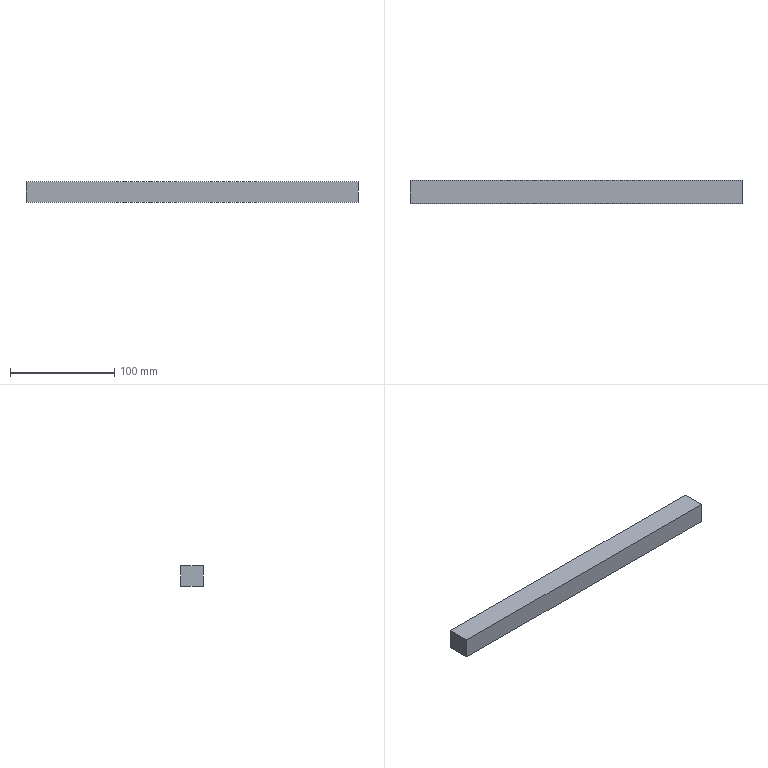Part | SolidWorks | features Extrusion 1 | 1 solid | 6 faces | box 318 x 22 x 20 mm | volume 139920 mm3 | plane 6
STEP:
#1=CARTESIAN_POINT('',(0.,22.,0.));
#2=VERTEX_POINT('',#1);
#3=CARTESIAN_POINT('',(0.,0.,0.));
#4=VERTEX_POINT('',#3);
#5=CARTESIAN_POINT('',(0.,0.,0.));
#6=DIRECTION('',(0.,-1.,0.));
#7=VECTOR('',#6,1000.);
#8=LINE('',#5,#7);
#9=EDGE_CURVE('',#2,#4,#8,.T.);
#10=ORIENTED_EDGE('',*,*,#9,.T.);
#11=CARTESIAN_POINT('',(0.,0.,20.));
#12=VERTEX_POINT('',#11);
#13=CARTESIAN_POINT('',(0.,0.,20.));
#14=DIRECTION('',(0.,0.,-1.));
#15=VECTOR('',#14,1000.);
#16=LINE('',#13,#15);
#17=EDGE_CURVE('',#12,#4,#16,.T.);
#18=ORIENTED_EDGE('',*,*,#17,.F.);
#19=CARTESIAN_POINT('',(0.,22.,20.));
#20=VERTEX_POINT('',#19);
#21=CARTESIAN_POINT('',(0.,0.,20.));
#22=DIRECTION('',(0.,-1.,0.));
#23=VECTOR('',#22,1000.);
#24=LINE('',#21,#23);
#25=EDGE_CURVE('',#20,#12,#24,.T.);
#26=ORIENTED_EDGE('',*,*,#25,.F.);
#27=CARTESIAN_POINT('',(0.,22.,20.));
#28=DIRECTION('',(0.,0.,-1.));
#29=VECTOR('',#28,1000.);
#30=LINE('',#27,#29);
#31=EDGE_CURVE('',#20,#2,#30,.T.);
#32=ORIENTED_EDGE('',*,*,#31,.T.);
#33=EDGE_LOOP('',(#10,#18,#26,#32));
#34=FACE_OUTER_BOUND('',#33,.T.);
#35=CARTESIAN_POINT('',(0.,0.,20.));
#36=DIRECTION('',(1.,0.,0.));
#37=DIRECTION('',(0.,0.,-1.));
#38=AXIS2_PLACEMENT_3D('',#35,#36,#37);
#39=PLANE('',#38);
#40=ADVANCED_FACE('',(#34),#39,.F.);
#41=CARTESIAN_POINT('',(318.,0.,0.));
#42=VERTEX_POINT('',#41);
#43=CARTESIAN_POINT('',(0.,0.,0.));
#44=DIRECTION('',(1.,0.,0.));
#45=VECTOR('',#44,1000.);
#46=LINE('',#43,#45);
#47=EDGE_CURVE('',#4,#42,#46,.T.);
#48=ORIENTED_EDGE('',*,*,#47,.T.);
#49=CARTESIAN_POINT('',(318.,0.,20.));
#50=VERTEX_POINT('',#49);
#51=CARTESIAN_POINT('',(318.,0.,20.));
#52=DIRECTION('',(0.,0.,-1.));
#53=VECTOR('',#52,1000.);
#54=LINE('',#51,#53);
#55=EDGE_CURVE('',#50,#42,#54,.T.);
#56=ORIENTED_EDGE('',*,*,#55,.F.);
#57=CARTESIAN_POINT('',(0.,0.,20.));
#58=DIRECTION('',(1.,0.,0.));
#59=VECTOR('',#58,1000.);
#60=LINE('',#57,#59);
#61=EDGE_CURVE('',#12,#50,#60,.T.);
#62=ORIENTED_EDGE('',*,*,#61,.F.);
#63=ORIENTED_EDGE('',*,*,#17,.T.);
#64=EDGE_LOOP('',(#48,#56,#62,#63));
#65=FACE_OUTER_BOUND('',#64,.T.);
#66=CARTESIAN_POINT('',(0.,0.,20.));
#67=DIRECTION('',(0.,1.,0.));
#68=DIRECTION('',(0.,0.,1.));
#69=AXIS2_PLACEMENT_3D('',#66,#67,#68);
#70=PLANE('',#69);
#71=ADVANCED_FACE('',(#65),#70,.F.);
#72=CARTESIAN_POINT('',(318.,22.,0.));
#73=VERTEX_POINT('',#72);
#74=CARTESIAN_POINT('',(318.,0.,0.));
#75=DIRECTION('',(0.,1.,0.));
#76=VECTOR('',#75,1000.);
#77=LINE('',#74,#76);
#78=EDGE_CURVE('',#42,#73,#77,.T.);
#79=ORIENTED_EDGE('',*,*,#78,.T.);
#80=CARTESIAN_POINT('',(318.,22.,20.));
#81=VERTEX_POINT('',#80);
#82=CARTESIAN_POINT('',(318.,22.,20.));
#83=DIRECTION('',(0.,0.,-1.));
#84=VECTOR('',#83,1000.);
#85=LINE('',#82,#84);
#86=EDGE_CURVE('',#81,#73,#85,.T.);
#87=ORIENTED_EDGE('',*,*,#86,.F.);
#88=CARTESIAN_POINT('',(318.,0.,20.));
#89=DIRECTION('',(0.,1.,0.));
#90=VECTOR('',#89,1000.);
#91=LINE('',#88,#90);
#92=EDGE_CURVE('',#50,#81,#91,.T.);
#93=ORIENTED_EDGE('',*,*,#92,.F.);
#94=ORIENTED_EDGE('',*,*,#55,.T.);
#95=EDGE_LOOP('',(#79,#87,#93,#94));
#96=FACE_OUTER_BOUND('',#95,.T.);
#97=CARTESIAN_POINT('',(318.,0.,20.));
#98=DIRECTION('',(-1.,0.,0.));
#99=DIRECTION('',(0.,0.,1.));
#100=AXIS2_PLACEMENT_3D('',#97,#98,#99);
#101=PLANE('',#100);
#102=ADVANCED_FACE('',(#96),#101,.F.);
#103=CARTESIAN_POINT('',(0.,22.,0.));
#104=DIRECTION('',(-1.,0.,0.));
#105=VECTOR('',#104,1000.);
#106=LINE('',#103,#105);
#107=EDGE_CURVE('',#73,#2,#106,.T.);
#108=ORIENTED_EDGE('',*,*,#107,.T.);
#109=ORIENTED_EDGE('',*,*,#31,.F.);
#110=CARTESIAN_POINT('',(0.,22.,20.));
#111=DIRECTION('',(-1.,0.,0.));
#112=VECTOR('',#111,1000.);
#113=LINE('',#110,#112);
#114=EDGE_CURVE('',#81,#20,#113,.T.);
#115=ORIENTED_EDGE('',*,*,#114,.F.);
#116=ORIENTED_EDGE('',*,*,#86,.T.);
#117=EDGE_LOOP('',(#108,#109,#115,#116));
#118=FACE_OUTER_BOUND('',#117,.T.);
#119=CARTESIAN_POINT('',(0.,22.,20.));
#120=DIRECTION('',(0.,-1.,0.));
#121=DIRECTION('',(0.,0.,-1.));
#122=AXIS2_PLACEMENT_3D('',#119,#120,#121);
#123=PLANE('',#122);
#124=ADVANCED_FACE('',(#118),#123,.F.);
#125=ORIENTED_EDGE('',*,*,#25,.T.);
#126=ORIENTED_EDGE('',*,*,#61,.T.);
#127=ORIENTED_EDGE('',*,*,#92,.T.);
#128=ORIENTED_EDGE('',*,*,#114,.T.);
#129=EDGE_LOOP('',(#125,#126,#127,#128));
#130=FACE_OUTER_BOUND('',#129,.T.);
#131=CARTESIAN_POINT('',(0.,0.,20.));
#132=DIRECTION('',(0.,0.,-1.));
#133=DIRECTION('',(-1.,0.,0.));
#134=AXIS2_PLACEMENT_3D('',#131,#132,#133);
#135=PLANE('',#134);
#136=ADVANCED_FACE('',(#130),#135,.F.);
#137=ORIENTED_EDGE('',*,*,#9,.F.);
#138=ORIENTED_EDGE('',*,*,#107,.F.);
#139=ORIENTED_EDGE('',*,*,#78,.F.);
#140=ORIENTED_EDGE('',*,*,#47,.F.);
#141=EDGE_LOOP('',(#137,#138,#139,#140));
#142=FACE_OUTER_BOUND('',#141,.T.);
#143=CARTESIAN_POINT('',(0.,0.,0.));
#144=DIRECTION('',(0.,0.,-1.));
#145=DIRECTION('',(-1.,0.,0.));
#146=AXIS2_PLACEMENT_3D('',#143,#144,#145);
#147=PLANE('',#146);
#148=ADVANCED_FACE('',(#142),#147,.T.);
#149=CLOSED_SHELL('',(#40,#71,#102,#124,#136,#148));
#150=MANIFOLD_SOLID_BREP('',#149);
#151=CARTESIAN_POINT('',(0.,0.,0.));
#152=DIRECTION('',(0.,0.,1.));
#153=DIRECTION('',(1.,0.,0.));
#154=AXIS2_PLACEMENT_3D('',#151,#152,#153);
#155=(LENGTH_UNIT()NAMED_UNIT(*)SI_UNIT(.MILLI.,.METRE.));
#156=UNCERTAINTY_MEASURE_WITH_UNIT(LENGTH_MEASURE(0.00001),#155,'','');
#157=(NAMED_UNIT(*)PLANE_ANGLE_UNIT()SI_UNIT($,.RADIAN.));
#158=(NAMED_UNIT(*)SI_UNIT($,.STERADIAN.)SOLID_ANGLE_UNIT());
#159=(GEOMETRIC_REPRESENTATION_CONTEXT(3)GLOBAL_UNCERTAINTY_ASSIGNED_CONTEXT((#156))GLOBAL_UNIT_ASSIGNED_CONTEXT((#155,#157,#158))REPRESENTATION_CONTEXT('',''));
#160=ADVANCED_BREP_SHAPE_REPRESENTATION('',(#150,#154),#159);